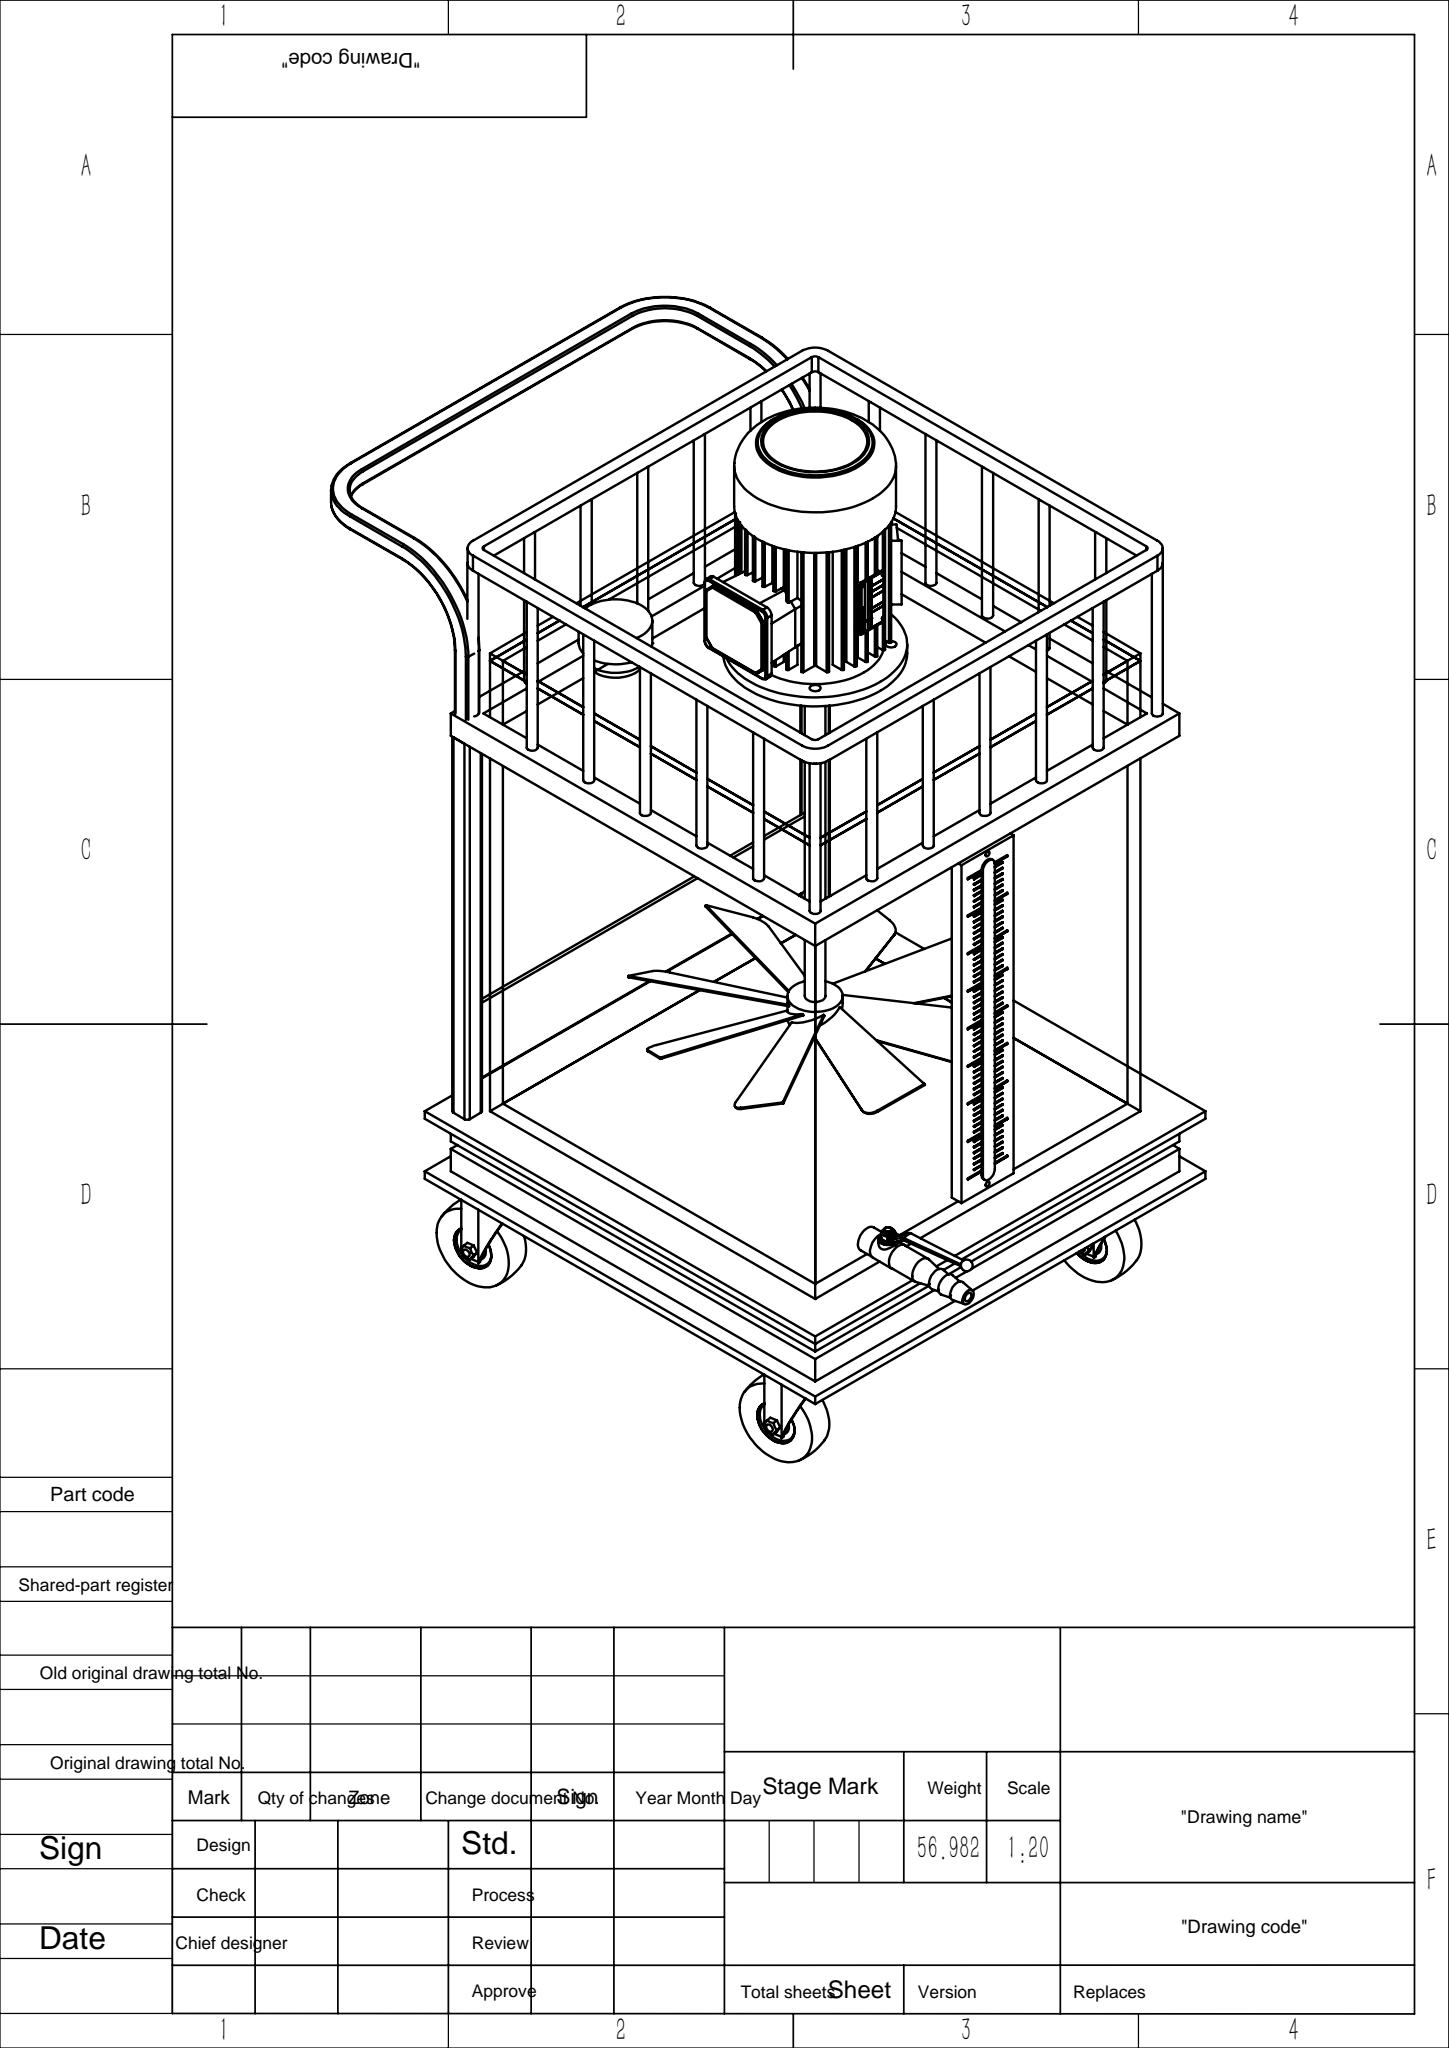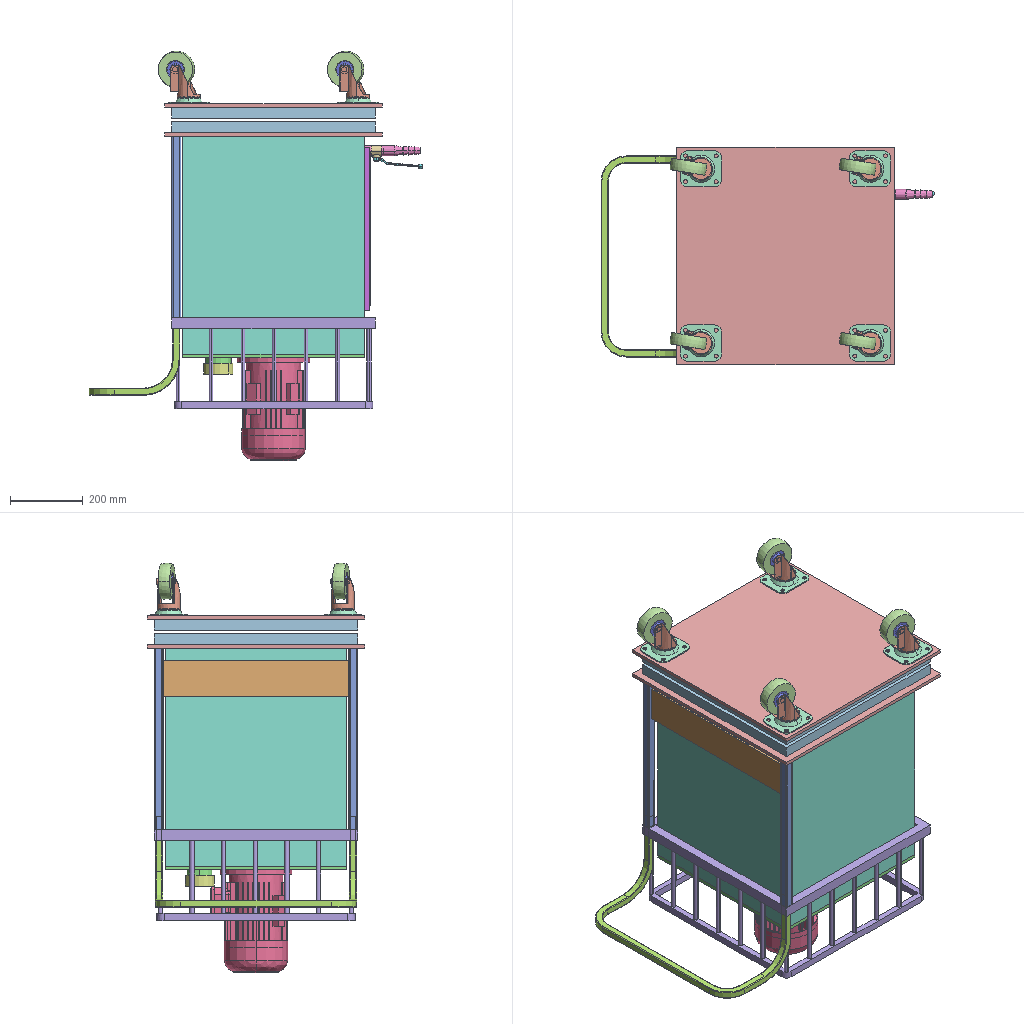Assembly | SolidWorks | 14 different items | 20 placed | box 919 x 600 x 1126 mm
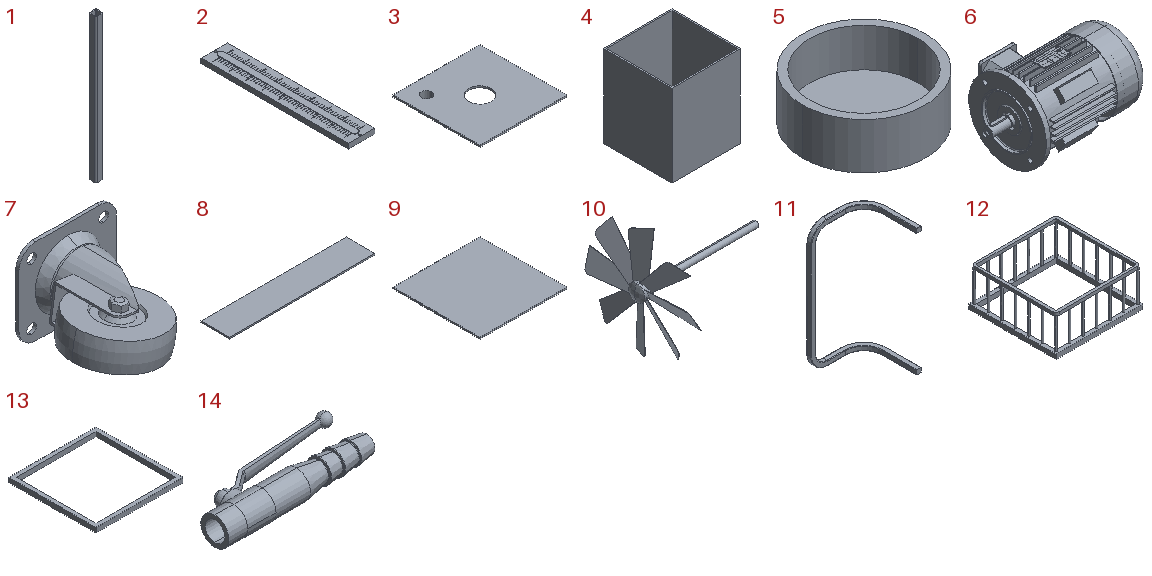Parts list (item | quantity | size | volume | features):
1 | x2 | 25 x 25 x 500 mm | 86850 mm3 | features Extrusion 1
2 | x1 | 80 x 450 x 17 mm | 554690 mm3 | features ICE 3, Extrusion 1, LPattern 1
3 | x1 | 500 x 500 x 50 mm | 2380238 mm3 | features Extrusion 1, ICE 1
4 | x1 | 500 x 500 x 600 mm | 14064000 mm3 | features Extrusion 1, Shell 1
5 | x1 | 80 x 80 x 30 mm | 54585 mm3 | features Extrusion 1, ICE 1
6 | x1 | 333 x 225 x 200 mm | 6079117 mm3 | features ICE 3, BaseBody 1
7 | x4 | - | - | features RefSurface 4
8 | x1 | 510 x 100 x 5 mm | 255000 mm3 | features Extrusion 1
9 | x2 | 600 x 600 x 10 mm | 3600000 mm3 | features Extrusion 1
10 | x1 | 444 x 407.086 x 407.086 mm | 372083 mm3 | features ICE 9, Revolution 3, CirPattern 2, Cut 1, Helix 1, RefAxis 1, Scale 1, SweepCut 1
11 | x1 | 250 x 250 x 554 mm | 533445 mm3 | features Fillet 3, Extrusion 1, ICE 1
12 | x1 | 560 x 560 x 250 mm | 2819829 mm3 | features ICE 2, Extrusion 1
13 | x2 | 560 x 560 x 30 mm | 1605000 mm3 | features Extrusion 1
14 | x1 | - | - | features ICE 2, RefSurface 2, Extrusion 1, Revolution 1, Scale 1
Mates (type | each side: item.copy, entity, surface, feature):
Coincident | 9.1 face plane Boss-Extrude1 | 7.1 face plane CMGJ100_R_swiwel-1-surface1
DistanceDim | 7.1 face plane CMGJ100_R_swiwel-1-surface1 | 9.1 face plane Boss-Extrude1
DistanceDim | 9.1 face plane Boss-Extrude1 | 7.1 face plane CMGJ100_R_swiwel-1-surface1
Coincident | 9.1 face plane Boss-Extrude1 | 7.2 face plane CMGJ100_R_swiwel-1-surface1
DistanceDim | 7.2 face plane CMGJ100_R_swiwel-1-surface1 | 9.1 face plane Boss-Extrude1
DistanceDim | 9.1 face plane Boss-Extrude1 | 7.2 face plane CMGJ100_R_swiwel-1-surface1
Coincident | 9.1 face plane Boss-Extrude1 | 7.3 face plane CMGJ100_R_swiwel-1-surface1
DistanceDim | 7.3 face plane CMGJ100_R_swiwel-1-surface1 | 9.1 face plane Boss-Extrude1 | 2 times
Coincident | 9.1 face plane Boss-Extrude1 | 7.4 face plane CMGJ100_R_swiwel-1-surface1
DistanceDim | 7.4 face plane CMGJ100_R_swiwel-1-surface1 | 9.1 face plane Boss-Extrude1 | 2 times
Coincident | 9.2 face plane Boss-Extrude1 | 1.1 face plane Boss-Extrude1
DistanceDim | 1.1 face plane Boss-Extrude1 | 9.1 face plane Boss-Extrude1 | 2 times
Coincident | 9.2 face plane Boss-Extrude1 | 1.2 face plane Boss-Extrude1
DistanceDim | 1.2 face plane Boss-Extrude1 | 9.1 face plane Boss-Extrude1 | 2 times
Coincident | 1.1 face plane Boss-Extrude1 | 11.1 face plane Cut-Extrude1
Coincident | 1.1 face plane Boss-Extrude1 | 11.1 face plane Boss-Extrude1
DistanceDim | 4.1 face plane Boss-Extrude1 | 9.1 face plane Boss-Extrude1 | 2 times
DistanceDim | 10.1 face cylinder Boss-Extrude5 | 4.1 face plane Boss-Extrude1 | 2 times
Coincident | 4.1 face plane Boss-Extrude1 | 14.1 face plane Boss-Extrude1
DistanceDim | 14.1 face cylinder Boss-Extrude1 | 4.1 face plane Boss-Extrude1
DistanceDim | 14.1 face cylinder Boss-Extrude1 | 9.2 face plane Boss-Extrude1
Coincident | 1.2 face plane Boss-Extrude1 | 8.1 face plane Boss-Extrude1
DistanceDim | 8.1 face plane Boss-Extrude1 | 1.2 face plane Boss-Extrude1
Coincident | 1.1 face plane Boss-Extrude1 | 12.1 face plane Boss-Extrude1 | 3 times
Coincident | 4.1 face plane Boss-Extrude1 | 3.1 face plane Boss-Extrude1 | 3 times
Coincident | 3.1 face plane Boss-Extrude1 | 6.1 face plane Input 1
Concentric | 3.1 face cylinder Boss-Extrude1 | 6.1 face cylinder Input 1
Parallel | 3.1 face plane Boss-Extrude1 | 6.1 face plane Input 1
Coincident | 10.1 face plane Boss-Extrude9 | 6.1 face plane Input 1
Coincident | 9.1 face plane Boss-Extrude1 | 13.1 face plane Boss-Extrude1
Coincident | 12.1 face plane Boss-Extrude1 | 13.1 face plane Boss-Extrude1
Coincident | 1.1 face plane Boss-Extrude1 | 13.1 face plane Boss-Extrude1
Coincident | 13.1 face plane Boss-Extrude1 | 13.2 face plane Boss-Extrude1 | 2 times
DistanceDim | 13.2 face plane Boss-Extrude1 | 13.1 face plane Boss-Extrude1
Coincident | 13.2 face plane Boss-Extrude1 | 9.2 face plane Boss-Extrude1
Coincident | 9.1 face plane Boss-Extrude1 | 9.2 face plane Boss-Extrude1 | 2 times
Coincident | 4.1 face plane Boss-Extrude1 | 9.2 face plane Boss-Extrude1
Coincident | 4.1 face plane Boss-Extrude1 | 2.1 face plane Boss-Extrude1
DistanceDim | 2.1 face plane Boss-Extrude1 | 9.2 face plane Boss-Extrude1
DistanceDim | 2.1 face plane Boss-Extrude1 | 4.1 face plane Boss-Extrude1
Concentric | 3.1 face cylinder Boss-Extrude2 | 5.1 face cylinder Boss-Extrude1
Coincident | 3.1 edge | 5.1 face plane Boss-Extrude1